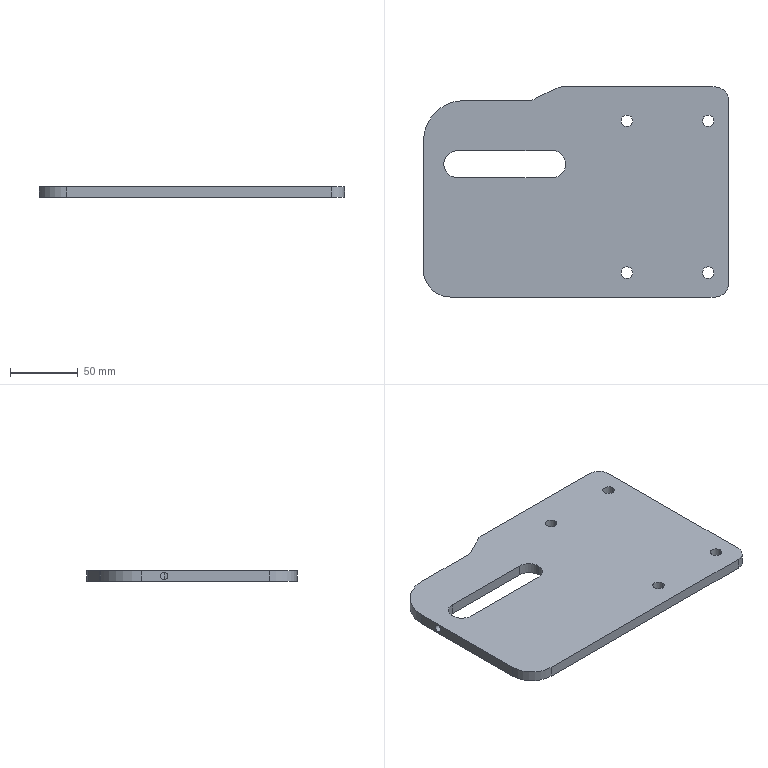Part | SolidWorks | features BaseBody 1 | 1 solid | 29 faces | box 225 x 155 x 8 mm | volume 253337 mm3 | cylinder 19 | plane 10 | commonest cylinder face diameters 8.5 x8 20 x7 5.5 x2 40 x1 60 x1
STEP:
#1=CARTESIAN_POINT('',(33.25,52.5,8.));
#2=VERTEX_POINT('',#1);
#3=CARTESIAN_POINT('',(41.75,52.5,8.));
#4=VERTEX_POINT('',#3);
#5=CARTESIAN_POINT('',(37.5,52.5,8.));
#6=DIRECTION('',(0.,0.,1.));
#7=DIRECTION('',(-1.,0.,0.));
#8=AXIS2_PLACEMENT_3D('',#5,#6,#7);
#9=CIRCLE('',#8,4.25);
#10=EDGE_CURVE('',#2,#4,#9,.T.);
#11=ORIENTED_EDGE('',*,*,#10,.T.);
#12=CARTESIAN_POINT('',(41.75,52.5,0.));
#13=VERTEX_POINT('',#12);
#14=CARTESIAN_POINT('',(41.75,52.5,0.));
#15=DIRECTION('',(0.,0.,-1.));
#16=VECTOR('',#15,1000.);
#17=LINE('',#14,#16);
#18=EDGE_CURVE('',#4,#13,#17,.T.);
#19=ORIENTED_EDGE('',*,*,#18,.T.);
#20=CARTESIAN_POINT('',(33.25,52.5,0.));
#21=VERTEX_POINT('',#20);
#22=CARTESIAN_POINT('',(37.5,52.5,0.));
#23=DIRECTION('',(0.,0.,1.));
#24=DIRECTION('',(-1.,0.,0.));
#25=AXIS2_PLACEMENT_3D('',#22,#23,#24);
#26=CIRCLE('',#25,4.25);
#27=EDGE_CURVE('',#21,#13,#26,.T.);
#28=ORIENTED_EDGE('',*,*,#27,.F.);
#29=CARTESIAN_POINT('',(33.25,52.5,0.));
#30=DIRECTION('',(0.,0.,-1.));
#31=VECTOR('',#30,1000.);
#32=LINE('',#29,#31);
#33=EDGE_CURVE('',#2,#21,#32,.T.);
#34=ORIENTED_EDGE('',*,*,#33,.F.);
#35=EDGE_LOOP('',(#11,#19,#28,#34));
#36=FACE_OUTER_BOUND('',#35,.T.);
#37=CARTESIAN_POINT('',(37.5,52.5,0.));
#38=DIRECTION('',(0.,0.,-1.));
#39=DIRECTION('',(-1.,0.,0.));
#40=AXIS2_PLACEMENT_3D('',#37,#38,#39);
#41=CYLINDRICAL_SURFACE('',#40,4.25);
#42=ADVANCED_FACE('',(#36),#41,.F.);
#43=CARTESIAN_POINT('',(93.25,-59.5,8.));
#44=VERTEX_POINT('',#43);
#45=CARTESIAN_POINT('',(101.75,-59.5,8.));
#46=VERTEX_POINT('',#45);
#47=CARTESIAN_POINT('',(97.5,-59.5,8.));
#48=DIRECTION('',(0.,0.,1.));
#49=DIRECTION('',(-1.,0.,0.));
#50=AXIS2_PLACEMENT_3D('',#47,#48,#49);
#51=CIRCLE('',#50,4.25);
#52=EDGE_CURVE('',#44,#46,#51,.T.);
#53=ORIENTED_EDGE('',*,*,#52,.T.);
#54=CARTESIAN_POINT('',(101.75,-59.5,0.));
#55=VERTEX_POINT('',#54);
#56=CARTESIAN_POINT('',(101.75,-59.5,0.));
#57=DIRECTION('',(0.,0.,-1.));
#58=VECTOR('',#57,1000.);
#59=LINE('',#56,#58);
#60=EDGE_CURVE('',#46,#55,#59,.T.);
#61=ORIENTED_EDGE('',*,*,#60,.T.);
#62=CARTESIAN_POINT('',(93.25,-59.5,0.));
#63=VERTEX_POINT('',#62);
#64=CARTESIAN_POINT('',(97.5,-59.5,0.));
#65=DIRECTION('',(0.,0.,1.));
#66=DIRECTION('',(-1.,0.,0.));
#67=AXIS2_PLACEMENT_3D('',#64,#65,#66);
#68=CIRCLE('',#67,4.25);
#69=EDGE_CURVE('',#63,#55,#68,.T.);
#70=ORIENTED_EDGE('',*,*,#69,.F.);
#71=CARTESIAN_POINT('',(93.25,-59.5,0.));
#72=DIRECTION('',(0.,0.,-1.));
#73=VECTOR('',#72,1000.);
#74=LINE('',#71,#73);
#75=EDGE_CURVE('',#44,#63,#74,.T.);
#76=ORIENTED_EDGE('',*,*,#75,.F.);
#77=EDGE_LOOP('',(#53,#61,#70,#76));
#78=FACE_OUTER_BOUND('',#77,.T.);
#79=CARTESIAN_POINT('',(97.5,-59.5,0.));
#80=DIRECTION('',(0.,0.,-1.));
#81=DIRECTION('',(-1.,0.,0.));
#82=AXIS2_PLACEMENT_3D('',#79,#80,#81);
#83=CYLINDRICAL_SURFACE('',#82,4.25);
#84=ADVANCED_FACE('',(#78),#83,.F.);
#85=CARTESIAN_POINT('',(33.25,-59.5,8.));
#86=VERTEX_POINT('',#85);
#87=CARTESIAN_POINT('',(41.75,-59.5,8.));
#88=VERTEX_POINT('',#87);
#89=CARTESIAN_POINT('',(37.5,-59.5,8.));
#90=DIRECTION('',(0.,0.,1.));
#91=DIRECTION('',(-1.,0.,0.));
#92=AXIS2_PLACEMENT_3D('',#89,#90,#91);
#93=CIRCLE('',#92,4.25);
#94=EDGE_CURVE('',#86,#88,#93,.T.);
#95=ORIENTED_EDGE('',*,*,#94,.T.);
#96=CARTESIAN_POINT('',(41.75,-59.5,0.));
#97=VERTEX_POINT('',#96);
#98=CARTESIAN_POINT('',(41.75,-59.5,0.));
#99=DIRECTION('',(0.,0.,-1.));
#100=VECTOR('',#99,1000.);
#101=LINE('',#98,#100);
#102=EDGE_CURVE('',#88,#97,#101,.T.);
#103=ORIENTED_EDGE('',*,*,#102,.T.);
#104=CARTESIAN_POINT('',(33.25,-59.5,0.));
#105=VERTEX_POINT('',#104);
#106=CARTESIAN_POINT('',(37.5,-59.5,0.));
#107=DIRECTION('',(0.,0.,1.));
#108=DIRECTION('',(-1.,0.,0.));
#109=AXIS2_PLACEMENT_3D('',#106,#107,#108);
#110=CIRCLE('',#109,4.25);
#111=EDGE_CURVE('',#105,#97,#110,.T.);
#112=ORIENTED_EDGE('',*,*,#111,.F.);
#113=CARTESIAN_POINT('',(33.25,-59.5,0.));
#114=DIRECTION('',(0.,0.,-1.));
#115=VECTOR('',#114,1000.);
#116=LINE('',#113,#115);
#117=EDGE_CURVE('',#86,#105,#116,.T.);
#118=ORIENTED_EDGE('',*,*,#117,.F.);
#119=EDGE_LOOP('',(#95,#103,#112,#118));
#120=FACE_OUTER_BOUND('',#119,.T.);
#121=CARTESIAN_POINT('',(37.5,-59.5,0.));
#122=DIRECTION('',(0.,0.,-1.));
#123=DIRECTION('',(-1.,0.,0.));
#124=AXIS2_PLACEMENT_3D('',#121,#122,#123);
#125=CYLINDRICAL_SURFACE('',#124,4.25);
#126=ADVANCED_FACE('',(#120),#125,.F.);
#127=CARTESIAN_POINT('',(93.25,52.5,8.));
#128=VERTEX_POINT('',#127);
#129=CARTESIAN_POINT('',(101.75,52.5,8.));
#130=VERTEX_POINT('',#129);
#131=CARTESIAN_POINT('',(97.5,52.5,8.));
#132=DIRECTION('',(0.,0.,1.));
#133=DIRECTION('',(-1.,0.,0.));
#134=AXIS2_PLACEMENT_3D('',#131,#132,#133);
#135=CIRCLE('',#134,4.25);
#136=EDGE_CURVE('',#128,#130,#135,.T.);
#137=ORIENTED_EDGE('',*,*,#136,.T.);
#138=CARTESIAN_POINT('',(101.75,52.5,0.));
#139=VERTEX_POINT('',#138);
#140=CARTESIAN_POINT('',(101.75,52.5,0.));
#141=DIRECTION('',(0.,0.,-1.));
#142=VECTOR('',#141,1000.);
#143=LINE('',#140,#142);
#144=EDGE_CURVE('',#130,#139,#143,.T.);
#145=ORIENTED_EDGE('',*,*,#144,.T.);
#146=CARTESIAN_POINT('',(93.25,52.5,0.));
#147=VERTEX_POINT('',#146);
#148=CARTESIAN_POINT('',(97.5,52.5,0.));
#149=DIRECTION('',(0.,0.,1.));
#150=DIRECTION('',(-1.,0.,0.));
#151=AXIS2_PLACEMENT_3D('',#148,#149,#150);
#152=CIRCLE('',#151,4.25);
#153=EDGE_CURVE('',#147,#139,#152,.T.);
#154=ORIENTED_EDGE('',*,*,#153,.F.);
#155=CARTESIAN_POINT('',(93.25,52.5,0.));
#156=DIRECTION('',(0.,0.,-1.));
#157=VECTOR('',#156,1000.);
#158=LINE('',#155,#157);
#159=EDGE_CURVE('',#128,#147,#158,.T.);
#160=ORIENTED_EDGE('',*,*,#159,.F.);
#161=EDGE_LOOP('',(#137,#145,#154,#160));
#162=FACE_OUTER_BOUND('',#161,.T.);
#163=CARTESIAN_POINT('',(97.5,52.5,0.));
#164=DIRECTION('',(0.,0.,-1.));
#165=DIRECTION('',(-1.,0.,0.));
#166=AXIS2_PLACEMENT_3D('',#163,#164,#165);
#167=CYLINDRICAL_SURFACE('',#166,4.25);
#168=ADVANCED_FACE('',(#162),#167,.F.);
#169=CARTESIAN_POINT('',(-7.5,20.5,0.));
#170=VERTEX_POINT('',#169);
#171=CARTESIAN_POINT('',(-17.5,30.5,0.));
#172=VERTEX_POINT('',#171);
#173=CARTESIAN_POINT('',(-17.5,20.5,0.));
#174=DIRECTION('',(0.,0.,1.));
#175=DIRECTION('',(1.,0.,0.));
#176=AXIS2_PLACEMENT_3D('',#173,#174,#175);
#177=CIRCLE('',#176,10.);
#178=EDGE_CURVE('',#170,#172,#177,.T.);
#179=ORIENTED_EDGE('',*,*,#178,.F.);
#180=CARTESIAN_POINT('',(-7.5,20.5,8.));
#181=VERTEX_POINT('',#180);
#182=CARTESIAN_POINT('',(-7.5,20.5,0.));
#183=DIRECTION('',(0.,0.,1.));
#184=VECTOR('',#183,1000.);
#185=LINE('',#182,#184);
#186=EDGE_CURVE('',#170,#181,#185,.T.);
#187=ORIENTED_EDGE('',*,*,#186,.T.);
#188=CARTESIAN_POINT('',(-17.5,30.5,8.));
#189=VERTEX_POINT('',#188);
#190=CARTESIAN_POINT('',(-17.5,20.5,8.));
#191=DIRECTION('',(0.,0.,1.));
#192=DIRECTION('',(1.,0.,0.));
#193=AXIS2_PLACEMENT_3D('',#190,#191,#192);
#194=CIRCLE('',#193,10.);
#195=EDGE_CURVE('',#181,#189,#194,.T.);
#196=ORIENTED_EDGE('',*,*,#195,.T.);
#197=CARTESIAN_POINT('',(-17.5,30.5,0.));
#198=DIRECTION('',(0.,0.,-1.));
#199=VECTOR('',#198,1000.);
#200=LINE('',#197,#199);
#201=EDGE_CURVE('',#189,#172,#200,.T.);
#202=ORIENTED_EDGE('',*,*,#201,.T.);
#203=EDGE_LOOP('',(#179,#187,#196,#202));
#204=FACE_OUTER_BOUND('',#203,.T.);
#205=CARTESIAN_POINT('',(-17.5,20.5,0.));
#206=DIRECTION('',(0.,0.,1.));
#207=DIRECTION('',(1.,0.,0.));
#208=AXIS2_PLACEMENT_3D('',#205,#206,#207);
#209=CYLINDRICAL_SURFACE('',#208,10.);
#210=ADVANCED_FACE('',(#204),#209,.F.);
#211=CARTESIAN_POINT('',(-97.5,20.5,6.75));
#212=VERTEX_POINT('',#211);
#213=CARTESIAN_POINT('',(-97.5,20.5,1.25));
#214=VERTEX_POINT('',#213);
#215=CARTESIAN_POINT('',(-97.5,20.5,6.75));
#216=CARTESIAN_POINT('',(-97.5,20.317,6.75));
#217=CARTESIAN_POINT('',(-97.495,20.138,6.732));
#218=CARTESIAN_POINT('',(-97.476,19.785,6.662));
#219=CARTESIAN_POINT('',(-97.462,19.61,6.608));
#220=CARTESIAN_POINT('',(-97.426,19.278,6.47));
#221=CARTESIAN_POINT('',(-97.405,19.12,6.386));
#222=CARTESIAN_POINT('',(-97.359,18.822,6.186));
#223=CARTESIAN_POINT('',(-97.334,18.681,6.071));
#224=CARTESIAN_POINT('',(-97.259,18.303,5.692));
#225=CARTESIAN_POINT('',(-97.208,18.099,5.387));
#226=CARTESIAN_POINT('',(-97.154,17.892,4.891));
#227=CARTESIAN_POINT('',(-97.14,17.839,4.717));
#228=CARTESIAN_POINT('',(-97.12,17.768,4.362));
#229=CARTESIAN_POINT('',(-97.114,17.75,4.183));
#230=CARTESIAN_POINT('',(-97.114,17.75,3.822));
#231=CARTESIAN_POINT('',(-97.12,17.768,3.639));
#232=CARTESIAN_POINT('',(-97.139,17.838,3.286));
#233=CARTESIAN_POINT('',(-97.154,17.89,3.114));
#234=CARTESIAN_POINT('',(-97.208,18.098,2.613));
#235=CARTESIAN_POINT('',(-97.259,18.3,2.311));
#236=CARTESIAN_POINT('',(-97.334,18.682,1.929));
#237=CARTESIAN_POINT('',(-97.359,18.819,1.816));
#238=CARTESIAN_POINT('',(-97.405,19.116,1.617));
#239=CARTESIAN_POINT('',(-97.426,19.277,1.53));
#240=CARTESIAN_POINT('',(-97.462,19.609,1.392));
#241=CARTESIAN_POINT('',(-97.476,19.78,1.34));
#242=CARTESIAN_POINT('',(-97.495,20.135,1.268));
#243=CARTESIAN_POINT('',(-97.5,20.317,1.25));
#244=CARTESIAN_POINT('',(-97.5,20.5,1.25));
#245=B_SPLINE_CURVE_WITH_KNOTS('',3,(#215,#216,#217,#218,#219,#220,#221,#222,#223,#224,#225,#226,#227,#228,#229,#230,#231,#232,#233,#234,#235,#236,#237,#238,#239,#240,#241,#242,#243,#244),.UNSPECIFIED.,.F.,.F.,(4,2,2,2,2,2,2,2,2,2,2,2,2,2,4),(0.008637,0.009177,0.009716,0.01026,0.0108,0.01188,0.01242,0.01295,0.01349,0.01403,0.01511,0.01565,0.01619,0.01673,0.01727),.UNSPECIFIED.);
#246=EDGE_CURVE('',#212,#214,#245,.T.);
#247=ORIENTED_EDGE('',*,*,#246,.T.);
#248=CARTESIAN_POINT('',(-112.5,20.5,1.25));
#249=VERTEX_POINT('',#248);
#250=CARTESIAN_POINT('',(-112.5,20.5,1.25));
#251=DIRECTION('',(-1.,0.,0.));
#252=VECTOR('',#251,1000.);
#253=LINE('',#250,#252);
#254=EDGE_CURVE('',#214,#249,#253,.T.);
#255=ORIENTED_EDGE('',*,*,#254,.T.);
#256=CARTESIAN_POINT('',(-112.5,20.5,6.75));
#257=VERTEX_POINT('',#256);
#258=CARTESIAN_POINT('',(-112.5,20.5,4.));
#259=DIRECTION('',(-1.,0.,0.));
#260=DIRECTION('',(0.,0.,1.));
#261=AXIS2_PLACEMENT_3D('',#258,#259,#260);
#262=CIRCLE('',#261,2.75);
#263=EDGE_CURVE('',#249,#257,#262,.T.);
#264=ORIENTED_EDGE('',*,*,#263,.T.);
#265=CARTESIAN_POINT('',(-112.5,20.5,6.75));
#266=DIRECTION('',(-1.,0.,0.));
#267=VECTOR('',#266,1000.);
#268=LINE('',#265,#267);
#269=EDGE_CURVE('',#212,#257,#268,.T.);
#270=ORIENTED_EDGE('',*,*,#269,.F.);
#271=EDGE_LOOP('',(#247,#255,#264,#270));
#272=FACE_OUTER_BOUND('',#271,.T.);
#273=CARTESIAN_POINT('',(-112.5,20.5,4.));
#274=DIRECTION('',(-1.,0.,0.));
#275=DIRECTION('',(0.,0.,1.));
#276=AXIS2_PLACEMENT_3D('',#273,#274,#275);
#277=CYLINDRICAL_SURFACE('',#276,2.75);
#278=ADVANCED_FACE('',(#272),#277,.F.);
#279=CARTESIAN_POINT('',(112.5,-67.5,8.));
#280=VERTEX_POINT('',#279);
#281=CARTESIAN_POINT('',(102.5,-77.5,8.));
#282=VERTEX_POINT('',#281);
#283=CARTESIAN_POINT('',(102.5,-67.5,8.));
#284=DIRECTION('',(0.,0.,-1.));
#285=DIRECTION('',(-1.,0.,0.));
#286=AXIS2_PLACEMENT_3D('',#283,#284,#285);
#287=CIRCLE('',#286,10.);
#288=EDGE_CURVE('',#280,#282,#287,.T.);
#289=ORIENTED_EDGE('',*,*,#288,.F.);
#290=CARTESIAN_POINT('',(112.5,67.5,8.));
#291=VERTEX_POINT('',#290);
#292=CARTESIAN_POINT('',(112.5,0.,8.));
#293=DIRECTION('',(0.,-1.,0.));
#294=VECTOR('',#293,1000.);
#295=LINE('',#292,#294);
#296=EDGE_CURVE('',#291,#280,#295,.T.);
#297=ORIENTED_EDGE('',*,*,#296,.F.);
#298=CARTESIAN_POINT('',(102.5,77.5,8.));
#299=VERTEX_POINT('',#298);
#300=CARTESIAN_POINT('',(102.5,67.5,8.));
#301=DIRECTION('',(0.,0.,-1.));
#302=DIRECTION('',(-1.,0.,0.));
#303=AXIS2_PLACEMENT_3D('',#300,#301,#302);
#304=CIRCLE('',#303,10.);
#305=EDGE_CURVE('',#299,#291,#304,.T.);
#306=ORIENTED_EDGE('',*,*,#305,.F.);
#307=CARTESIAN_POINT('',(-10.139,77.5,8.));
#308=VERTEX_POINT('',#307);
#309=CARTESIAN_POINT('',(0.,77.5,8.));
#310=DIRECTION('',(1.,0.,0.));
#311=VECTOR('',#310,1000.);
#312=LINE('',#309,#311);
#313=EDGE_CURVE('',#308,#299,#312,.T.);
#314=ORIENTED_EDGE('',*,*,#313,.F.);
#315=CARTESIAN_POINT('',(-14.611,76.444,8.));
#316=VERTEX_POINT('',#315);
#317=CARTESIAN_POINT('',(-10.139,67.5,8.));
#318=DIRECTION('',(0.,0.,-1.));
#319=DIRECTION('',(-1.,0.,0.));
#320=AXIS2_PLACEMENT_3D('',#317,#318,#319);
#321=CIRCLE('',#320,10.);
#322=EDGE_CURVE('',#316,#308,#321,.T.);
#323=ORIENTED_EDGE('',*,*,#322,.F.);
#324=CARTESIAN_POINT('',(-30.389,68.556,8.));
#325=VERTEX_POINT('',#324);
#326=CARTESIAN_POINT('',(-30.389,68.556,8.));
#327=DIRECTION('',(0.8944,0.4472,0.));
#328=VECTOR('',#327,1000.);
#329=LINE('',#326,#328);
#330=EDGE_CURVE('',#325,#316,#329,.T.);
#331=ORIENTED_EDGE('',*,*,#330,.F.);
#332=CARTESIAN_POINT('',(-34.861,67.5,8.));
#333=VERTEX_POINT('',#332);
#334=CARTESIAN_POINT('',(-34.861,77.5,8.));
#335=DIRECTION('',(0.,0.,1.));
#336=DIRECTION('',(1.,0.,0.));
#337=AXIS2_PLACEMENT_3D('',#334,#335,#336);
#338=CIRCLE('',#337,10.);
#339=EDGE_CURVE('',#333,#325,#338,.T.);
#340=ORIENTED_EDGE('',*,*,#339,.F.);
#341=CARTESIAN_POINT('',(-82.5,67.5,8.));
#342=VERTEX_POINT('',#341);
#343=CARTESIAN_POINT('',(0.,67.5,8.));
#344=DIRECTION('',(1.,0.,0.));
#345=VECTOR('',#344,1000.);
#346=LINE('',#343,#345);
#347=EDGE_CURVE('',#342,#333,#346,.T.);
#348=ORIENTED_EDGE('',*,*,#347,.F.);
#349=CARTESIAN_POINT('',(-112.5,37.5,8.));
#350=VERTEX_POINT('',#349);
#351=CARTESIAN_POINT('',(-82.5,37.5,8.));
#352=DIRECTION('',(0.,0.,-1.));
#353=DIRECTION('',(-1.,0.,0.));
#354=AXIS2_PLACEMENT_3D('',#351,#352,#353);
#355=CIRCLE('',#354,30.);
#356=EDGE_CURVE('',#350,#342,#355,.T.);
#357=ORIENTED_EDGE('',*,*,#356,.F.);
#358=CARTESIAN_POINT('',(-112.5,-57.5,8.));
#359=VERTEX_POINT('',#358);
#360=CARTESIAN_POINT('',(-112.5,0.,8.));
#361=DIRECTION('',(0.,1.,0.));
#362=VECTOR('',#361,1000.);
#363=LINE('',#360,#362);
#364=EDGE_CURVE('',#359,#350,#363,.T.);
#365=ORIENTED_EDGE('',*,*,#364,.F.);
#366=CARTESIAN_POINT('',(-92.5,-77.5,8.));
#367=VERTEX_POINT('',#366);
#368=CARTESIAN_POINT('',(-92.5,-57.5,8.));
#369=DIRECTION('',(0.,0.,-1.));
#370=DIRECTION('',(-1.,0.,0.));
#371=AXIS2_PLACEMENT_3D('',#368,#369,#370);
#372=CIRCLE('',#371,20.);
#373=EDGE_CURVE('',#367,#359,#372,.T.);
#374=ORIENTED_EDGE('',*,*,#373,.F.);
#375=CARTESIAN_POINT('',(0.,-77.5,8.));
#376=DIRECTION('',(-1.,0.,0.));
#377=VECTOR('',#376,1000.);
#378=LINE('',#375,#377);
#379=EDGE_CURVE('',#282,#367,#378,.T.);
#380=ORIENTED_EDGE('',*,*,#379,.F.);
#381=EDGE_LOOP('',(#289,#297,#306,#314,#323,#331,#340,#348,#357,#365,#374,#380));
#382=FACE_OUTER_BOUND('',#381,.T.);
#383=ORIENTED_EDGE('',*,*,#10,.F.);
#384=CARTESIAN_POINT('',(37.5,52.5,8.));
#385=DIRECTION('',(0.,0.,1.));
#386=DIRECTION('',(-1.,0.,0.));
#387=AXIS2_PLACEMENT_3D('',#384,#385,#386);
#388=CIRCLE('',#387,4.25);
#389=EDGE_CURVE('',#4,#2,#388,.T.);
#390=ORIENTED_EDGE('',*,*,#389,.F.);
#391=EDGE_LOOP('',(#383,#390));
#392=FACE_BOUND('',#391,.T.);
#393=ORIENTED_EDGE('',*,*,#52,.F.);
#394=CARTESIAN_POINT('',(97.5,-59.5,8.));
#395=DIRECTION('',(0.,0.,1.));
#396=DIRECTION('',(-1.,0.,0.));
#397=AXIS2_PLACEMENT_3D('',#394,#395,#396);
#398=CIRCLE('',#397,4.25);
#399=EDGE_CURVE('',#46,#44,#398,.T.);
#400=ORIENTED_EDGE('',*,*,#399,.F.);
#401=EDGE_LOOP('',(#393,#400));
#402=FACE_BOUND('',#401,.T.);
#403=ORIENTED_EDGE('',*,*,#94,.F.);
#404=CARTESIAN_POINT('',(37.5,-59.5,8.));
#405=DIRECTION('',(0.,0.,1.));
#406=DIRECTION('',(-1.,0.,0.));
#407=AXIS2_PLACEMENT_3D('',#404,#405,#406);
#408=CIRCLE('',#407,4.25);
#409=EDGE_CURVE('',#88,#86,#408,.T.);
#410=ORIENTED_EDGE('',*,*,#409,.F.);
#411=EDGE_LOOP('',(#403,#410));
#412=FACE_BOUND('',#411,.T.);
#413=ORIENTED_EDGE('',*,*,#136,.F.);
#414=CARTESIAN_POINT('',(97.5,52.5,8.));
#415=DIRECTION('',(0.,0.,1.));
#416=DIRECTION('',(-1.,0.,0.));
#417=AXIS2_PLACEMENT_3D('',#414,#415,#416);
#418=CIRCLE('',#417,4.25);
#419=EDGE_CURVE('',#130,#128,#418,.T.);
#420=ORIENTED_EDGE('',*,*,#419,.F.);
#421=EDGE_LOOP('',(#413,#420));
#422=FACE_BOUND('',#421,.T.);
#423=CARTESIAN_POINT('',(-87.5,30.5,8.));
#424=VERTEX_POINT('',#423);
#425=CARTESIAN_POINT('',(-87.5,10.5,8.));
#426=VERTEX_POINT('',#425);
#427=CARTESIAN_POINT('',(-87.5,20.5,8.));
#428=DIRECTION('',(0.,0.,1.));
#429=DIRECTION('',(1.,0.,0.));
#430=AXIS2_PLACEMENT_3D('',#427,#428,#429);
#431=CIRCLE('',#430,10.);
#432=EDGE_CURVE('',#424,#426,#431,.T.);
#433=ORIENTED_EDGE('',*,*,#432,.F.);
#434=CARTESIAN_POINT('',(0.,30.5,8.));
#435=DIRECTION('',(-1.,0.,0.));
#436=VECTOR('',#435,1000.);
#437=LINE('',#434,#436);
#438=EDGE_CURVE('',#189,#424,#437,.T.);
#439=ORIENTED_EDGE('',*,*,#438,.F.);
#440=ORIENTED_EDGE('',*,*,#195,.F.);
#441=CARTESIAN_POINT('',(-17.5,10.5,8.));
#442=VERTEX_POINT('',#441);
#443=CARTESIAN_POINT('',(-17.5,20.5,8.));
#444=DIRECTION('',(0.,0.,1.));
#445=DIRECTION('',(1.,0.,0.));
#446=AXIS2_PLACEMENT_3D('',#443,#444,#445);
#447=CIRCLE('',#446,10.);
#448=EDGE_CURVE('',#442,#181,#447,.T.);
#449=ORIENTED_EDGE('',*,*,#448,.F.);
#450=CARTESIAN_POINT('',(0.,10.5,8.));
#451=DIRECTION('',(1.,0.,0.));
#452=VECTOR('',#451,1000.);
#453=LINE('',#450,#452);
#454=EDGE_CURVE('',#426,#442,#453,.T.);
#455=ORIENTED_EDGE('',*,*,#454,.F.);
#456=EDGE_LOOP('',(#433,#439,#440,#449,#455));
#457=FACE_BOUND('',#456,.T.);
#458=CARTESIAN_POINT('',(0.,0.,8.));
#459=DIRECTION('',(0.,0.,-1.));
#460=DIRECTION('',(-1.,0.,0.));
#461=AXIS2_PLACEMENT_3D('',#458,#459,#460);
#462=PLANE('',#461);
#463=ADVANCED_FACE('',(#382,#392,#402,#412,#422,#457),#462,.F.);
#464=CARTESIAN_POINT('',(102.5,-77.5,0.));
#465=VERTEX_POINT('',#464);
#466=CARTESIAN_POINT('',(102.5,-77.5,8.));
#467=DIRECTION('',(0.,0.,-1.));
#468=VECTOR('',#467,1000.);
#469=LINE('',#466,#468);
#470=EDGE_CURVE('',#282,#465,#469,.T.);
#471=ORIENTED_EDGE('',*,*,#470,.F.);
#472=ORIENTED_EDGE('',*,*,#379,.T.);
#473=CARTESIAN_POINT('',(-92.5,-77.5,0.));
#474=VERTEX_POINT('',#473);
#475=CARTESIAN_POINT('',(-92.5,-77.5,8.));
#476=DIRECTION('',(0.,0.,1.));
#477=VECTOR('',#476,1000.);
#478=LINE('',#475,#477);
#479=EDGE_CURVE('',#474,#367,#478,.T.);
#480=ORIENTED_EDGE('',*,*,#479,.F.);
#481=CARTESIAN_POINT('',(-112.5,-77.5,0.));
#482=DIRECTION('',(-1.,0.,0.));
#483=VECTOR('',#482,1000.);
#484=LINE('',#481,#483);
#485=EDGE_CURVE('',#465,#474,#484,.T.);
#486=ORIENTED_EDGE('',*,*,#485,.F.);
#487=EDGE_LOOP('',(#471,#472,#480,#486));
#488=FACE_OUTER_BOUND('',#487,.T.);
#489=CARTESIAN_POINT('',(-112.5,-77.5,8.));
#490=DIRECTION('',(0.,1.,0.));
#491=DIRECTION('',(0.,0.,1.));
#492=AXIS2_PLACEMENT_3D('',#489,#490,#491);
#493=PLANE('',#492);
#494=ADVANCED_FACE('',(#488),#493,.F.);
#495=CARTESIAN_POINT('',(112.5,-67.5,0.));
#496=VERTEX_POINT('',#495);
#497=CARTESIAN_POINT('',(102.5,-67.5,0.));
#498=DIRECTION('',(0.,0.,1.));
#499=DIRECTION('',(-1.,0.,0.));
#500=AXIS2_PLACEMENT_3D('',#497,#498,#499);
#501=CIRCLE('',#500,10.);
#502=EDGE_CURVE('',#465,#496,#501,.T.);
#503=ORIENTED_EDGE('',*,*,#502,.T.);
#504=CARTESIAN_POINT('',(112.5,-67.5,8.));
#505=DIRECTION('',(0.,0.,1.));
#506=VECTOR('',#505,1000.);
#507=LINE('',#504,#506);
#508=EDGE_CURVE('',#496,#280,#507,.T.);
#509=ORIENTED_EDGE('',*,*,#508,.T.);
#510=ORIENTED_EDGE('',*,*,#288,.T.);
#511=ORIENTED_EDGE('',*,*,#470,.T.);
#512=EDGE_LOOP('',(#503,#509,#510,#511));
#513=FACE_OUTER_BOUND('',#512,.T.);
#514=CARTESIAN_POINT('',(102.5,-67.5,8.));
#515=DIRECTION('',(0.,0.,-1.));
#516=DIRECTION('',(-1.,0.,0.));
#517=AXIS2_PLACEMENT_3D('',#514,#515,#516);
#518=CYLINDRICAL_SURFACE('',#517,10.);
#519=ADVANCED_FACE('',(#513),#518,.T.);
#520=ORIENTED_EDGE('',*,*,#508,.F.);
#521=CARTESIAN_POINT('',(112.5,67.5,0.));
#522=VERTEX_POINT('',#521);
#523=CARTESIAN_POINT('',(112.5,-77.5,0.));
#524=DIRECTION('',(0.,-1.,0.));
#525=VECTOR('',#524,1000.);
#526=LINE('',#523,#525);
#527=EDGE_CURVE('',#522,#496,#526,.T.);
#528=ORIENTED_EDGE('',*,*,#527,.F.);
#529=CARTESIAN_POINT('',(112.5,67.5,8.));
#530=DIRECTION('',(0.,0.,-1.));
#531=VECTOR('',#530,1000.);
#532=LINE('',#529,#531);
#533=EDGE_CURVE('',#291,#522,#532,.T.);
#534=ORIENTED_EDGE('',*,*,#533,.F.);
#535=ORIENTED_EDGE('',*,*,#296,.T.);
#536=EDGE_LOOP('',(#520,#528,#534,#535));
#537=FACE_OUTER_BOUND('',#536,.T.);
#538=CARTESIAN_POINT('',(112.5,-77.5,8.));
#539=DIRECTION('',(-1.,0.,0.));
#540=DIRECTION('',(0.,0.,1.));
#541=AXIS2_PLACEMENT_3D('',#538,#539,#540);
#542=PLANE('',#541);
#543=ADVANCED_FACE('',(#537),#542,.F.);
#544=CARTESIAN_POINT('',(102.5,77.5,0.));
#545=VERTEX_POINT('',#544);
#546=CARTESIAN_POINT('',(102.5,67.5,0.));
#547=DIRECTION('',(0.,0.,1.));
#548=DIRECTION('',(-1.,0.,0.));
#549=AXIS2_PLACEMENT_3D('',#546,#547,#548);
#550=CIRCLE('',#549,10.);
#551=EDGE_CURVE('',#522,#545,#550,.T.);
#552=ORIENTED_EDGE('',*,*,#551,.T.);
#553=CARTESIAN_POINT('',(102.5,77.5,8.));
#554=DIRECTION('',(0.,0.,1.));
#555=VECTOR('',#554,1000.);
#556=LINE('',#553,#555);
#557=EDGE_CURVE('',#545,#299,#556,.T.);
#558=ORIENTED_EDGE('',*,*,#557,.T.);
#559=ORIENTED_EDGE('',*,*,#305,.T.);
#560=ORIENTED_EDGE('',*,*,#533,.T.);
#561=EDGE_LOOP('',(#552,#558,#559,#560));
#562=FACE_OUTER_BOUND('',#561,.T.);
#563=CARTESIAN_POINT('',(102.5,67.5,8.));
#564=DIRECTION('',(0.,0.,-1.));
#565=DIRECTION('',(-1.,0.,0.));
#566=AXIS2_PLACEMENT_3D('',#563,#564,#565);
#567=CYLINDRICAL_SURFACE('',#566,10.);
#568=ADVANCED_FACE('',(#562),#567,.T.);
#569=ORIENTED_EDGE('',*,*,#557,.F.);
#570=CARTESIAN_POINT('',(-10.139,77.5,0.));
#571=VERTEX_POINT('',#570);
#572=CARTESIAN_POINT('',(-112.5,77.5,0.));
#573=DIRECTION('',(1.,0.,0.));
#574=VECTOR('',#573,1000.);
#575=LINE('',#572,#574);
#576=EDGE_CURVE('',#571,#545,#575,.T.);
#577=ORIENTED_EDGE('',*,*,#576,.F.);
#578=CARTESIAN_POINT('',(-10.139,77.5,8.));
#579=DIRECTION('',(0.,0.,-1.));
#580=VECTOR('',#579,1000.);
#581=LINE('',#578,#580);
#582=EDGE_CURVE('',#308,#571,#581,.T.);
#583=ORIENTED_EDGE('',*,*,#582,.F.);
#584=ORIENTED_EDGE('',*,*,#313,.T.);
#585=EDGE_LOOP('',(#569,#577,#583,#584));
#586=FACE_OUTER_BOUND('',#585,.T.);
#587=CARTESIAN_POINT('',(-112.5,77.5,8.));
#588=DIRECTION('',(0.,-1.,0.));
#589=DIRECTION('',(0.,0.,-1.));
#590=AXIS2_PLACEMENT_3D('',#587,#588,#589);
#591=PLANE('',#590);
#592=ADVANCED_FACE('',(#586),#591,.F.);
#593=CARTESIAN_POINT('',(-14.611,76.444,0.));
#594=VERTEX_POINT('',#593);
#595=CARTESIAN_POINT('',(-10.139,67.5,0.));
#596=DIRECTION('',(0.,0.,1.));
#597=DIRECTION('',(-1.,0.,0.));
#598=AXIS2_PLACEMENT_3D('',#595,#596,#597);
#599=CIRCLE('',#598,10.);
#600=EDGE_CURVE('',#571,#594,#599,.T.);
#601=ORIENTED_EDGE('',*,*,#600,.T.);
#602=CARTESIAN_POINT('',(-14.611,76.444,8.));
#603=DIRECTION('',(0.,0.,1.));
#604=VECTOR('',#603,1000.);
#605=LINE('',#602,#604);
#606=EDGE_CURVE('',#594,#316,#605,.T.);
#607=ORIENTED_EDGE('',*,*,#606,.T.);
#608=ORIENTED_EDGE('',*,*,#322,.T.);
#609=ORIENTED_EDGE('',*,*,#582,.T.);
#610=EDGE_LOOP('',(#601,#607,#608,#609));
#611=FACE_OUTER_BOUND('',#610,.T.);
#612=CARTESIAN_POINT('',(-10.139,67.5,8.));
#613=DIRECTION('',(0.,0.,-1.));
#614=DIRECTION('',(-1.,0.,0.));
#615=AXIS2_PLACEMENT_3D('',#612,#613,#614);
#616=CYLINDRICAL_SURFACE('',#615,10.);
#617=ADVANCED_FACE('',(#611),#616,.T.);
#618=CARTESIAN_POINT('',(-30.389,68.556,0.));
#619=VERTEX_POINT('',#618);
#620=CARTESIAN_POINT('',(-30.389,68.556,8.));
#621=DIRECTION('',(0.,0.,-1.));
#622=VECTOR('',#621,1000.);
#623=LINE('',#620,#622);
#624=EDGE_CURVE('',#325,#619,#623,.T.);
#625=ORIENTED_EDGE('',*,*,#624,.F.);
#626=ORIENTED_EDGE('',*,*,#330,.T.);
#627=ORIENTED_EDGE('',*,*,#606,.F.);
#628=CARTESIAN_POINT('',(-32.5,67.5,0.));
#629=DIRECTION('',(0.8944,0.4472,0.));
#630=VECTOR('',#629,1000.);
#631=LINE('',#628,#630);
#632=EDGE_CURVE('',#619,#594,#631,.T.);
#633=ORIENTED_EDGE('',*,*,#632,.F.);
#634=EDGE_LOOP('',(#625,#626,#627,#633));
#635=FACE_OUTER_BOUND('',#634,.T.);
#636=CARTESIAN_POINT('',(-32.5,67.5,8.));
#637=DIRECTION('',(0.4472,-0.8944,0.));
#638=DIRECTION('',(0.8944,0.4472,0.));
#639=AXIS2_PLACEMENT_3D('',#636,#637,#638);
#640=PLANE('',#639);
#641=ADVANCED_FACE('',(#635),#640,.F.);
#642=ORIENTED_EDGE('',*,*,#624,.T.);
#643=CARTESIAN_POINT('',(-34.861,67.5,0.));
#644=VERTEX_POINT('',#643);
#645=CARTESIAN_POINT('',(-34.861,77.5,0.));
#646=DIRECTION('',(0.,0.,1.));
#647=DIRECTION('',(1.,0.,0.));
#648=AXIS2_PLACEMENT_3D('',#645,#646,#647);
#649=CIRCLE('',#648,10.);
#650=EDGE_CURVE('',#644,#619,#649,.T.);
#651=ORIENTED_EDGE('',*,*,#650,.F.);
#652=CARTESIAN_POINT('',(-34.861,67.5,8.));
#653=DIRECTION('',(0.,0.,-1.));
#654=VECTOR('',#653,1000.);
#655=LINE('',#652,#654);
#656=EDGE_CURVE('',#333,#644,#655,.T.);
#657=ORIENTED_EDGE('',*,*,#656,.F.);
#658=ORIENTED_EDGE('',*,*,#339,.T.);
#659=EDGE_LOOP('',(#642,#651,#657,#658));
#660=FACE_OUTER_BOUND('',#659,.T.);
#661=CARTESIAN_POINT('',(-34.861,77.5,8.));
#662=DIRECTION('',(0.,0.,1.));
#663=DIRECTION('',(1.,0.,0.));
#664=AXIS2_PLACEMENT_3D('',#661,#662,#663);
#665=CYLINDRICAL_SURFACE('',#664,10.);
#666=ADVANCED_FACE('',(#660),#665,.F.);
#667=ORIENTED_EDGE('',*,*,#656,.T.);
#668=CARTESIAN_POINT('',(-82.5,67.5,0.));
#669=VERTEX_POINT('',#668);
#670=CARTESIAN_POINT('',(-112.5,67.5,0.));
#671=DIRECTION('',(1.,0.,0.));
#672=VECTOR('',#671,1000.);
#673=LINE('',#670,#672);
#674=EDGE_CURVE('',#669,#644,#673,.T.);
#675=ORIENTED_EDGE('',*,*,#674,.F.);
#676=CARTESIAN_POINT('',(-82.5,67.5,8.));
#677=DIRECTION('',(0.,0.,-1.));
#678=VECTOR('',#677,1000.);
#679=LINE('',#676,#678);
#680=EDGE_CURVE('',#342,#669,#679,.T.);
#681=ORIENTED_EDGE('',*,*,#680,.F.);
#682=ORIENTED_EDGE('',*,*,#347,.T.);
#683=EDGE_LOOP('',(#667,#675,#681,#682));
#684=FACE_OUTER_BOUND('',#683,.T.);
#685=CARTESIAN_POINT('',(-112.5,67.5,8.));
#686=DIRECTION('',(0.,-1.,0.));
#687=DIRECTION('',(1.,0.,0.));
#688=AXIS2_PLACEMENT_3D('',#685,#686,#687);
#689=PLANE('',#688);
#690=ADVANCED_FACE('',(#684),#689,.F.);
#691=CARTESIAN_POINT('',(-112.5,37.5,0.));
#692=VERTEX_POINT('',#691);
#693=CARTESIAN_POINT('',(-82.5,37.5,0.));
#694=DIRECTION('',(0.,0.,1.));
#695=DIRECTION('',(-1.,0.,0.));
#696=AXIS2_PLACEMENT_3D('',#693,#694,#695);
#697=CIRCLE('',#696,30.);
#698=EDGE_CURVE('',#669,#692,#697,.T.);
#699=ORIENTED_EDGE('',*,*,#698,.T.);
#700=CARTESIAN_POINT('',(-112.5,37.5,8.));
#701=DIRECTION('',(0.,0.,1.));
#702=VECTOR('',#701,1000.);
#703=LINE('',#700,#702);
#704=EDGE_CURVE('',#692,#350,#703,.T.);
#705=ORIENTED_EDGE('',*,*,#704,.T.);
#706=ORIENTED_EDGE('',*,*,#356,.T.);
#707=ORIENTED_EDGE('',*,*,#680,.T.);
#708=EDGE_LOOP('',(#699,#705,#706,#707));
#709=FACE_OUTER_BOUND('',#708,.T.);
#710=CARTESIAN_POINT('',(-82.5,37.5,8.));
#711=DIRECTION('',(0.,0.,-1.));
#712=DIRECTION('',(-1.,0.,0.));
#713=AXIS2_PLACEMENT_3D('',#710,#711,#712);
#714=CYLINDRICAL_SURFACE('',#713,30.);
#715=ADVANCED_FACE('',(#709),#714,.T.);
#716=CARTESIAN_POINT('',(-112.5,-57.5,0.));
#717=VERTEX_POINT('',#716);
#718=CARTESIAN_POINT('',(-112.5,-57.5,8.));
#719=DIRECTION('',(0.,0.,-1.));
#720=VECTOR('',#719,1000.);
#721=LINE('',#718,#720);
#722=EDGE_CURVE('',#359,#717,#721,.T.);
#723=ORIENTED_EDGE('',*,*,#722,.F.);
#724=ORIENTED_EDGE('',*,*,#364,.T.);
#725=ORIENTED_EDGE('',*,*,#704,.F.);
#726=CARTESIAN_POINT('',(-112.5,-77.5,0.));
#727=DIRECTION('',(0.,1.,0.));
#728=VECTOR('',#727,1000.);
#729=LINE('',#726,#728);
#730=EDGE_CURVE('',#717,#692,#729,.T.);
#731=ORIENTED_EDGE('',*,*,#730,.F.);
#732=EDGE_LOOP('',(#723,#724,#725,#731));
#733=FACE_OUTER_BOUND('',#732,.T.);
#734=CARTESIAN_POINT('',(-112.5,20.5,4.));
#735=DIRECTION('',(-1.,0.,0.));
#736=DIRECTION('',(0.,0.,1.));
#737=AXIS2_PLACEMENT_3D('',#734,#735,#736);
#738=CIRCLE('',#737,2.75);
#739=EDGE_CURVE('',#257,#249,#738,.T.);
#740=ORIENTED_EDGE('',*,*,#739,.F.);
#741=ORIENTED_EDGE('',*,*,#263,.F.);
#742=EDGE_LOOP('',(#740,#741));
#743=FACE_BOUND('',#742,.T.);
#744=CARTESIAN_POINT('',(-112.5,-77.5,8.));
#745=DIRECTION('',(1.,0.,0.));
#746=DIRECTION('',(0.,0.,-1.));
#747=AXIS2_PLACEMENT_3D('',#744,#745,#746);
#748=PLANE('',#747);
#749=ADVANCED_FACE('',(#733,#743),#748,.F.);
#750=CARTESIAN_POINT('',(-92.5,-57.5,0.));
#751=DIRECTION('',(0.,0.,1.));
#752=DIRECTION('',(-1.,0.,0.));
#753=AXIS2_PLACEMENT_3D('',#750,#751,#752);
#754=CIRCLE('',#753,20.);
#755=EDGE_CURVE('',#717,#474,#754,.T.);
#756=ORIENTED_EDGE('',*,*,#755,.T.);
#757=ORIENTED_EDGE('',*,*,#479,.T.);
#758=ORIENTED_EDGE('',*,*,#373,.T.);
#759=ORIENTED_EDGE('',*,*,#722,.T.);
#760=EDGE_LOOP('',(#756,#757,#758,#759));
#761=FACE_OUTER_BOUND('',#760,.T.);
#762=CARTESIAN_POINT('',(-92.5,-57.5,8.));
#763=DIRECTION('',(0.,0.,-1.));
#764=DIRECTION('',(-1.,0.,0.));
#765=AXIS2_PLACEMENT_3D('',#762,#763,#764);
#766=CYLINDRICAL_SURFACE('',#765,20.);
#767=ADVANCED_FACE('',(#761),#766,.T.);
#768=ORIENTED_EDGE('',*,*,#18,.F.);
#769=ORIENTED_EDGE('',*,*,#389,.T.);
#770=ORIENTED_EDGE('',*,*,#33,.T.);
#771=CARTESIAN_POINT('',(37.5,52.5,0.));
#772=DIRECTION('',(0.,0.,1.));
#773=DIRECTION('',(-1.,0.,0.));
#774=AXIS2_PLACEMENT_3D('',#771,#772,#773);
#775=CIRCLE('',#774,4.25);
#776=EDGE_CURVE('',#13,#21,#775,.T.);
#777=ORIENTED_EDGE('',*,*,#776,.F.);
#778=EDGE_LOOP('',(#768,#769,#770,#777));
#779=FACE_OUTER_BOUND('',#778,.T.);
#780=CARTESIAN_POINT('',(37.5,52.5,0.));
#781=DIRECTION('',(0.,0.,-1.));
#782=DIRECTION('',(-1.,0.,0.));
#783=AXIS2_PLACEMENT_3D('',#780,#781,#782);
#784=CYLINDRICAL_SURFACE('',#783,4.25);
#785=ADVANCED_FACE('',(#779),#784,.F.);
#786=ORIENTED_EDGE('',*,*,#60,.F.);
#787=ORIENTED_EDGE('',*,*,#399,.T.);
#788=ORIENTED_EDGE('',*,*,#75,.T.);
#789=CARTESIAN_POINT('',(97.5,-59.5,0.));
#790=DIRECTION('',(0.,0.,1.));
#791=DIRECTION('',(-1.,0.,0.));
#792=AXIS2_PLACEMENT_3D('',#789,#790,#791);
#793=CIRCLE('',#792,4.25);
#794=EDGE_CURVE('',#55,#63,#793,.T.);
#795=ORIENTED_EDGE('',*,*,#794,.F.);
#796=EDGE_LOOP('',(#786,#787,#788,#795));
#797=FACE_OUTER_BOUND('',#796,.T.);
#798=CARTESIAN_POINT('',(97.5,-59.5,0.));
#799=DIRECTION('',(0.,0.,-1.));
#800=DIRECTION('',(-1.,0.,0.));
#801=AXIS2_PLACEMENT_3D('',#798,#799,#800);
#802=CYLINDRICAL_SURFACE('',#801,4.25);
#803=ADVANCED_FACE('',(#797),#802,.F.);
#804=ORIENTED_EDGE('',*,*,#102,.F.);
#805=ORIENTED_EDGE('',*,*,#409,.T.);
#806=ORIENTED_EDGE('',*,*,#117,.T.);
#807=CARTESIAN_POINT('',(37.5,-59.5,0.));
#808=DIRECTION('',(0.,0.,1.));
#809=DIRECTION('',(-1.,0.,0.));
#810=AXIS2_PLACEMENT_3D('',#807,#808,#809);
#811=CIRCLE('',#810,4.25);
#812=EDGE_CURVE('',#97,#105,#811,.T.);
#813=ORIENTED_EDGE('',*,*,#812,.F.);
#814=EDGE_LOOP('',(#804,#805,#806,#813));
#815=FACE_OUTER_BOUND('',#814,.T.);
#816=CARTESIAN_POINT('',(37.5,-59.5,0.));
#817=DIRECTION('',(0.,0.,-1.));
#818=DIRECTION('',(-1.,0.,0.));
#819=AXIS2_PLACEMENT_3D('',#816,#817,#818);
#820=CYLINDRICAL_SURFACE('',#819,4.25);
#821=ADVANCED_FACE('',(#815),#820,.F.);
#822=ORIENTED_EDGE('',*,*,#144,.F.);
#823=ORIENTED_EDGE('',*,*,#419,.T.);
#824=ORIENTED_EDGE('',*,*,#159,.T.);
#825=CARTESIAN_POINT('',(97.5,52.5,0.));
#826=DIRECTION('',(0.,0.,1.));
#827=DIRECTION('',(-1.,0.,0.));
#828=AXIS2_PLACEMENT_3D('',#825,#826,#827);
#829=CIRCLE('',#828,4.25);
#830=EDGE_CURVE('',#139,#147,#829,.T.);
#831=ORIENTED_EDGE('',*,*,#830,.F.);
#832=EDGE_LOOP('',(#822,#823,#824,#831));
#833=FACE_OUTER_BOUND('',#832,.T.);
#834=CARTESIAN_POINT('',(97.5,52.5,0.));
#835=DIRECTION('',(0.,0.,-1.));
#836=DIRECTION('',(-1.,0.,0.));
#837=AXIS2_PLACEMENT_3D('',#834,#835,#836);
#838=CYLINDRICAL_SURFACE('',#837,4.25);
#839=ADVANCED_FACE('',(#833),#838,.F.);
#840=CARTESIAN_POINT('',(-17.5,10.5,0.));
#841=VERTEX_POINT('',#840);
#842=CARTESIAN_POINT('',(-17.5,10.5,0.));
#843=DIRECTION('',(0.,0.,1.));
#844=VECTOR('',#843,1000.);
#845=LINE('',#842,#844);
#846=EDGE_CURVE('',#841,#442,#845,.T.);
#847=ORIENTED_EDGE('',*,*,#846,.F.);
#848=CARTESIAN_POINT('',(-87.5,10.5,0.));
#849=VERTEX_POINT('',#848);
#850=CARTESIAN_POINT('',(-87.5,10.5,0.));
#851=DIRECTION('',(1.,0.,0.));
#852=VECTOR('',#851,1000.);
#853=LINE('',#850,#852);
#854=EDGE_CURVE('',#849,#841,#853,.T.);
#855=ORIENTED_EDGE('',*,*,#854,.F.);
#856=CARTESIAN_POINT('',(-87.5,10.5,0.));
#857=DIRECTION('',(0.,0.,-1.));
#858=VECTOR('',#857,1000.);
#859=LINE('',#856,#858);
#860=EDGE_CURVE('',#426,#849,#859,.T.);
#861=ORIENTED_EDGE('',*,*,#860,.F.);
#862=ORIENTED_EDGE('',*,*,#454,.T.);
#863=EDGE_LOOP('',(#847,#855,#861,#862));
#864=FACE_OUTER_BOUND('',#863,.T.);
#865=CARTESIAN_POINT('',(-87.5,10.5,0.));
#866=DIRECTION('',(0.,-1.,0.));
#867=DIRECTION('',(0.,0.,-1.));
#868=AXIS2_PLACEMENT_3D('',#865,#866,#867);
#869=PLANE('',#868);
#870=ADVANCED_FACE('',(#864),#869,.F.);
#871=ORIENTED_EDGE('',*,*,#860,.T.);
#872=CARTESIAN_POINT('',(-87.5,30.5,0.));
#873=VERTEX_POINT('',#872);
#874=CARTESIAN_POINT('',(-87.5,20.5,0.));
#875=DIRECTION('',(0.,0.,1.));
#876=DIRECTION('',(1.,0.,0.));
#877=AXIS2_PLACEMENT_3D('',#874,#875,#876);
#878=CIRCLE('',#877,10.);
#879=EDGE_CURVE('',#873,#849,#878,.T.);
#880=ORIENTED_EDGE('',*,*,#879,.F.);
#881=CARTESIAN_POINT('',(-87.5,30.5,0.));
#882=DIRECTION('',(0.,0.,-1.));
#883=VECTOR('',#882,1000.);
#884=LINE('',#881,#883);
#885=EDGE_CURVE('',#424,#873,#884,.T.);
#886=ORIENTED_EDGE('',*,*,#885,.F.);
#887=ORIENTED_EDGE('',*,*,#432,.T.);
#888=EDGE_LOOP('',(#871,#880,#886,#887));
#889=FACE_OUTER_BOUND('',#888,.T.);
#890=ORIENTED_EDGE('',*,*,#246,.F.);
#891=CARTESIAN_POINT('',(-97.5,20.5,1.25));
#892=CARTESIAN_POINT('',(-97.5,20.683,1.25));
#893=CARTESIAN_POINT('',(-97.495,20.862,1.268));
#894=CARTESIAN_POINT('',(-97.476,21.215,1.338));
#895=CARTESIAN_POINT('',(-97.462,21.39,1.392));
#896=CARTESIAN_POINT('',(-97.426,21.722,1.53));
#897=CARTESIAN_POINT('',(-97.405,21.88,1.614));
#898=CARTESIAN_POINT('',(-97.359,22.178,1.814));
#899=CARTESIAN_POINT('',(-97.334,22.319,1.929));
#900=CARTESIAN_POINT('',(-97.259,22.697,2.308));
#901=CARTESIAN_POINT('',(-97.208,22.901,2.613));
#902=CARTESIAN_POINT('',(-97.154,23.108,3.109));
#903=CARTESIAN_POINT('',(-97.14,23.161,3.283));
#904=CARTESIAN_POINT('',(-97.12,23.232,3.638));
#905=CARTESIAN_POINT('',(-97.114,23.25,3.817));
#906=CARTESIAN_POINT('',(-97.114,23.25,4.178));
#907=CARTESIAN_POINT('',(-97.12,23.232,4.361));
#908=CARTESIAN_POINT('',(-97.139,23.162,4.714));
#909=CARTESIAN_POINT('',(-97.154,23.11,4.886));
#910=CARTESIAN_POINT('',(-97.208,22.902,5.387));
#911=CARTESIAN_POINT('',(-97.259,22.7,5.689));
#912=CARTESIAN_POINT('',(-97.334,22.318,6.071));
#913=CARTESIAN_POINT('',(-97.359,22.181,6.184));
#914=CARTESIAN_POINT('',(-97.405,21.884,6.383));
#915=CARTESIAN_POINT('',(-97.426,21.723,6.47));
#916=CARTESIAN_POINT('',(-97.462,21.391,6.608));
#917=CARTESIAN_POINT('',(-97.476,21.22,6.66));
#918=CARTESIAN_POINT('',(-97.495,20.865,6.732));
#919=CARTESIAN_POINT('',(-97.5,20.683,6.75));
#920=CARTESIAN_POINT('',(-97.5,20.5,6.75));
#921=B_SPLINE_CURVE_WITH_KNOTS('',3,(#891,#892,#893,#894,#895,#896,#897,#898,#899,#900,#901,#902,#903,#904,#905,#906,#907,#908,#909,#910,#911,#912,#913,#914,#915,#916,#917,#918,#919,#920),.UNSPECIFIED.,.F.,.F.,(4,2,2,2,2,2,2,2,2,2,2,2,2,2,4),(0.,0.0005398,0.00108,0.001619,0.002159,0.003239,0.003779,0.004318,0.004858,0.005398,0.006478,0.007017,0.007557,0.008097,0.008637),.UNSPECIFIED.);
#922=EDGE_CURVE('',#214,#212,#921,.T.);
#923=ORIENTED_EDGE('',*,*,#922,.F.);
#924=EDGE_LOOP('',(#890,#923));
#925=FACE_BOUND('',#924,.T.);
#926=CARTESIAN_POINT('',(-87.5,20.5,0.));
#927=DIRECTION('',(0.,0.,1.));
#928=DIRECTION('',(1.,0.,0.));
#929=AXIS2_PLACEMENT_3D('',#926,#927,#928);
#930=CYLINDRICAL_SURFACE('',#929,10.);
#931=ADVANCED_FACE('',(#889,#925),#930,.F.);
#932=ORIENTED_EDGE('',*,*,#885,.T.);
#933=CARTESIAN_POINT('',(-87.5,30.5,0.));
#934=DIRECTION('',(-1.,0.,0.));
#935=VECTOR('',#934,1000.);
#936=LINE('',#933,#935);
#937=EDGE_CURVE('',#172,#873,#936,.T.);
#938=ORIENTED_EDGE('',*,*,#937,.F.);
#939=ORIENTED_EDGE('',*,*,#201,.F.);
#940=ORIENTED_EDGE('',*,*,#438,.T.);
#941=EDGE_LOOP('',(#932,#938,#939,#940));
#942=FACE_OUTER_BOUND('',#941,.T.);
#943=CARTESIAN_POINT('',(-87.5,30.5,0.));
#944=DIRECTION('',(0.,1.,0.));
#945=DIRECTION('',(0.,0.,1.));
#946=AXIS2_PLACEMENT_3D('',#943,#944,#945);
#947=PLANE('',#946);
#948=ADVANCED_FACE('',(#942),#947,.F.);
#949=ORIENTED_EDGE('',*,*,#186,.F.);
#950=CARTESIAN_POINT('',(-17.5,20.5,0.));
#951=DIRECTION('',(0.,0.,1.));
#952=DIRECTION('',(1.,0.,0.));
#953=AXIS2_PLACEMENT_3D('',#950,#951,#952);
#954=CIRCLE('',#953,10.);
#955=EDGE_CURVE('',#841,#170,#954,.T.);
#956=ORIENTED_EDGE('',*,*,#955,.F.);
#957=ORIENTED_EDGE('',*,*,#846,.T.);
#958=ORIENTED_EDGE('',*,*,#448,.T.);
#959=EDGE_LOOP('',(#949,#956,#957,#958));
#960=FACE_OUTER_BOUND('',#959,.T.);
#961=CARTESIAN_POINT('',(-17.5,20.5,0.));
#962=DIRECTION('',(0.,0.,1.));
#963=DIRECTION('',(1.,0.,0.));
#964=AXIS2_PLACEMENT_3D('',#961,#962,#963);
#965=CYLINDRICAL_SURFACE('',#964,10.);
#966=ADVANCED_FACE('',(#960),#965,.F.);
#967=ORIENTED_EDGE('',*,*,#576,.T.);
#968=ORIENTED_EDGE('',*,*,#551,.F.);
#969=ORIENTED_EDGE('',*,*,#527,.T.);
#970=ORIENTED_EDGE('',*,*,#502,.F.);
#971=ORIENTED_EDGE('',*,*,#485,.T.);
#972=ORIENTED_EDGE('',*,*,#755,.F.);
#973=ORIENTED_EDGE('',*,*,#730,.T.);
#974=ORIENTED_EDGE('',*,*,#698,.F.);
#975=ORIENTED_EDGE('',*,*,#674,.T.);
#976=ORIENTED_EDGE('',*,*,#650,.T.);
#977=ORIENTED_EDGE('',*,*,#632,.T.);
#978=ORIENTED_EDGE('',*,*,#600,.F.);
#979=EDGE_LOOP('',(#967,#968,#969,#970,#971,#972,#973,#974,#975,#976,#977,#978));
#980=FACE_OUTER_BOUND('',#979,.T.);
#981=ORIENTED_EDGE('',*,*,#27,.T.);
#982=ORIENTED_EDGE('',*,*,#776,.T.);
#983=EDGE_LOOP('',(#981,#982));
#984=FACE_BOUND('',#983,.T.);
#985=ORIENTED_EDGE('',*,*,#69,.T.);
#986=ORIENTED_EDGE('',*,*,#794,.T.);
#987=EDGE_LOOP('',(#985,#986));
#988=FACE_BOUND('',#987,.T.);
#989=ORIENTED_EDGE('',*,*,#111,.T.);
#990=ORIENTED_EDGE('',*,*,#812,.T.);
#991=EDGE_LOOP('',(#989,#990));
#992=FACE_BOUND('',#991,.T.);
#993=ORIENTED_EDGE('',*,*,#153,.T.);
#994=ORIENTED_EDGE('',*,*,#830,.T.);
#995=EDGE_LOOP('',(#993,#994));
#996=FACE_BOUND('',#995,.T.);
#997=ORIENTED_EDGE('',*,*,#955,.T.);
#998=ORIENTED_EDGE('',*,*,#178,.T.);
#999=ORIENTED_EDGE('',*,*,#937,.T.);
#1000=ORIENTED_EDGE('',*,*,#879,.T.);
#1001=ORIENTED_EDGE('',*,*,#854,.T.);
#1002=EDGE_LOOP('',(#997,#998,#999,#1000,#1001));
#1003=FACE_BOUND('',#1002,.T.);
#1004=CARTESIAN_POINT('',(0.,0.,0.));
#1005=DIRECTION('',(0.,0.,-1.));
#1006=DIRECTION('',(-1.,0.,0.));
#1007=AXIS2_PLACEMENT_3D('',#1004,#1005,#1006);
#1008=PLANE('',#1007);
#1009=ADVANCED_FACE('',(#980,#984,#988,#992,#996,#1003),#1008,.T.);
#1010=ORIENTED_EDGE('',*,*,#254,.F.);
#1011=ORIENTED_EDGE('',*,*,#922,.T.);
#1012=ORIENTED_EDGE('',*,*,#269,.T.);
#1013=ORIENTED_EDGE('',*,*,#739,.T.);
#1014=EDGE_LOOP('',(#1010,#1011,#1012,#1013));
#1015=FACE_OUTER_BOUND('',#1014,.T.);
#1016=CARTESIAN_POINT('',(-112.5,20.5,4.));
#1017=DIRECTION('',(-1.,0.,0.));
#1018=DIRECTION('',(0.,0.,1.));
#1019=AXIS2_PLACEMENT_3D('',#1016,#1017,#1018);
#1020=CYLINDRICAL_SURFACE('',#1019,2.75);
#1021=ADVANCED_FACE('',(#1015),#1020,.F.);
#1022=CLOSED_SHELL('',(#42,#84,#126,#168,#210,#278,#463,#494,#519,#543,#568,#592,#617,#641,#666,#690,#715,#749,#767,#785,#803,#821,#839,#870,#931,#948,#966,#1009,#1021));
#1023=MANIFOLD_SOLID_BREP('',#1022);
#1024=CARTESIAN_POINT('',(0.,0.,0.));
#1025=DIRECTION('',(0.,0.,1.));
#1026=DIRECTION('',(1.,0.,0.));
#1027=AXIS2_PLACEMENT_3D('',#1024,#1025,#1026);
#1028=(LENGTH_UNIT()NAMED_UNIT(*)SI_UNIT(.MILLI.,.METRE.));
#1029=UNCERTAINTY_MEASURE_WITH_UNIT(LENGTH_MEASURE(0.00001),#1028,'','');
#1030=(NAMED_UNIT(*)PLANE_ANGLE_UNIT()SI_UNIT($,.RADIAN.));
#1031=(NAMED_UNIT(*)SI_UNIT($,.STERADIAN.)SOLID_ANGLE_UNIT());
#1032=(GEOMETRIC_REPRESENTATION_CONTEXT(3)GLOBAL_UNCERTAINTY_ASSIGNED_CONTEXT((#1029))GLOBAL_UNIT_ASSIGNED_CONTEXT((#1028,#1030,#1031))REPRESENTATION_CONTEXT('',''));
#1033=ADVANCED_BREP_SHAPE_REPRESENTATION('',(#1023,#1027),#1032);